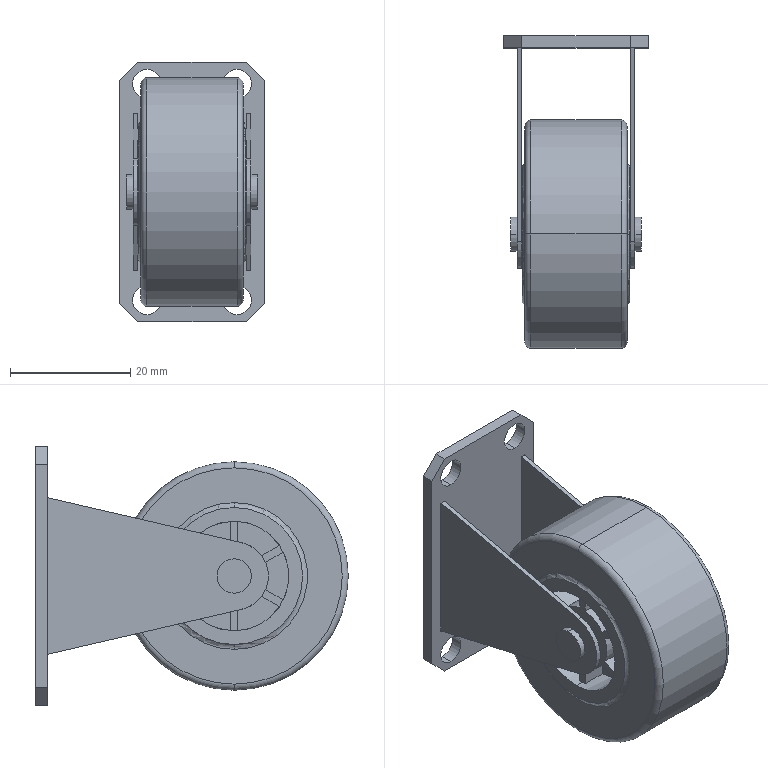Part | NX | features BREP 1, DATUM_CSYS 1 | 1 solid | 111 faces | box 24 x 52 x 43.2 mm | volume 20648 mm3 | plane 63 | cylinder 38 | torus 10 | commonest cylinder face diameters 11.4 x14 4.8 x8 5.7 x8 18.24 x4 14.4 x2 38 x2